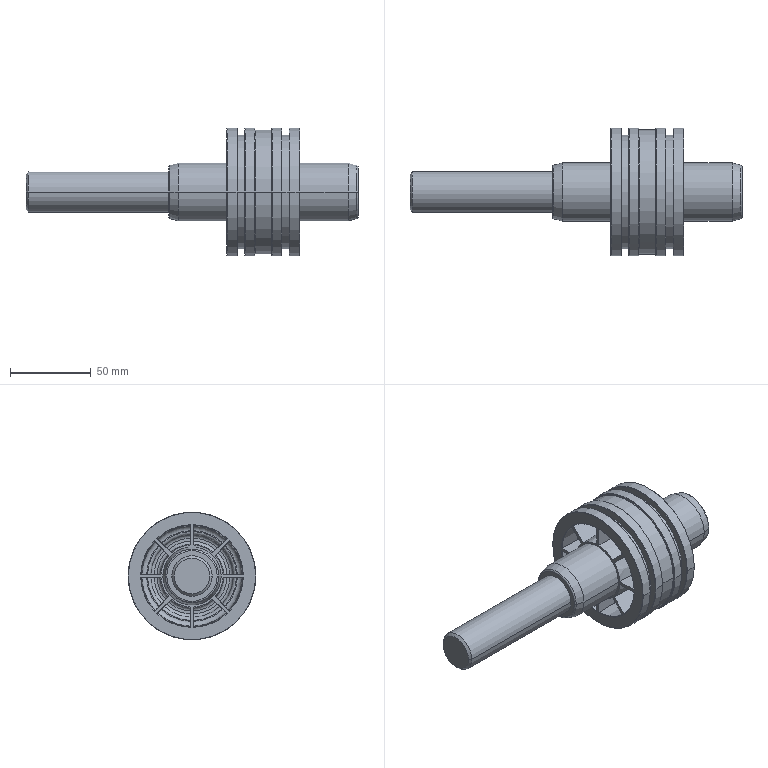Part | STEP file | SCT_80x100x25_r2 | 1 solid | 242 faces | box 205 x 79 x 79 mm | volume 224494 mm3 | plane 76 | torus 74 | cone 72 | cylinder 20 | commonest cylinder face diameters 79 x8 36 x4 70 x4 25 x2 76.9 x2